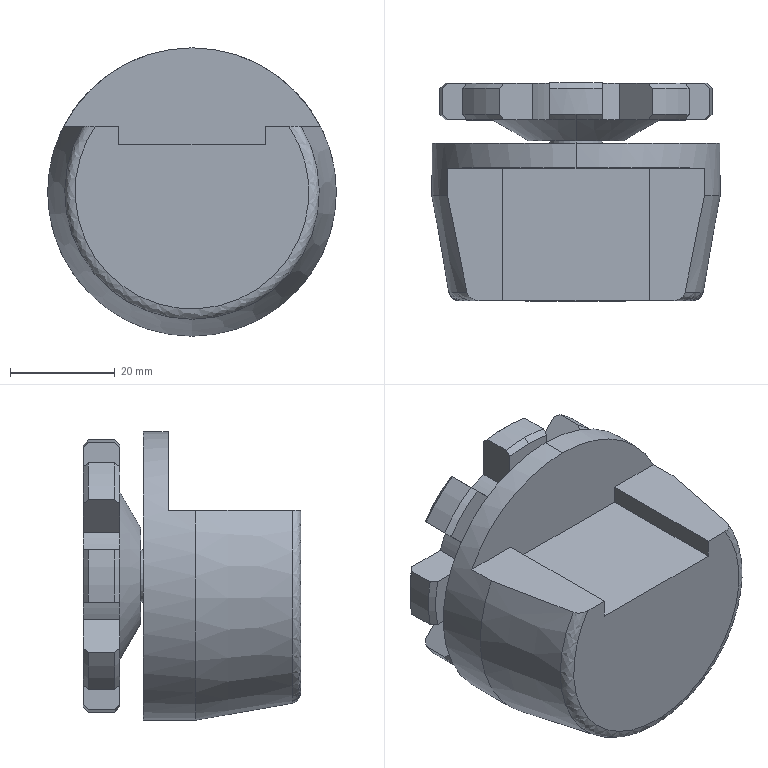Part | STEP file | _CGR01-60-U-004_1 | 1 solid | 85 faces | box 55 x 41.5 x 55 mm | volume 64973 mm3 | plane 31 | cylinder 27 | cone 26 | spline 1 | commonest cylinder face diameters 52 x9 35 x8 10 x4 4.134 x2 8.376 x2 55 x2